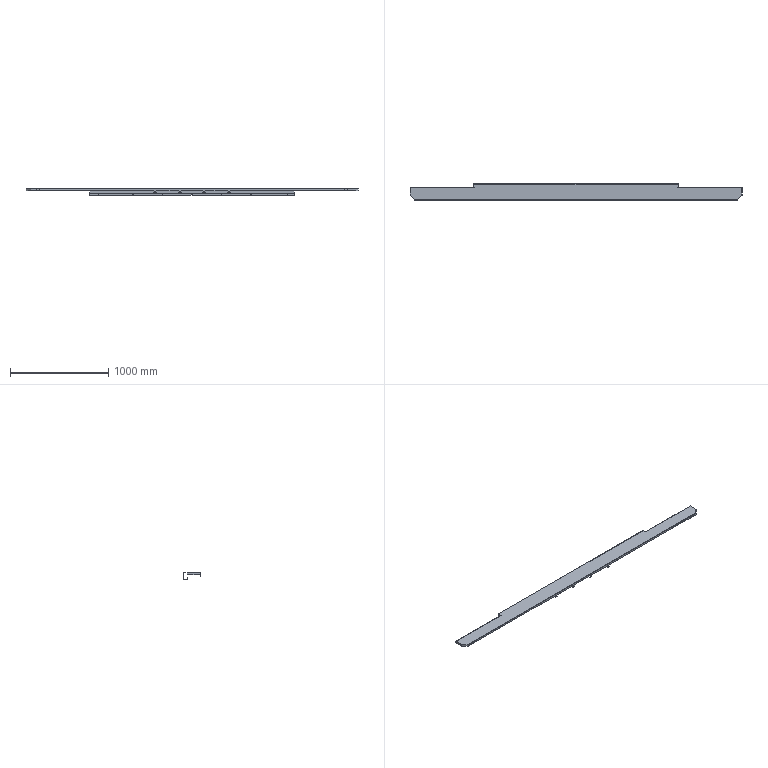Part | NX | features BREP 1 | 1 solid | 188 faces | box 3380 x 166 x 69 mm | volume 1251743 mm3 | plane 96 | cylinder 80 | spline 12 | commonest cylinder face diameters 4.2 x28 6 x18 10 x14 4 x10 7 x10